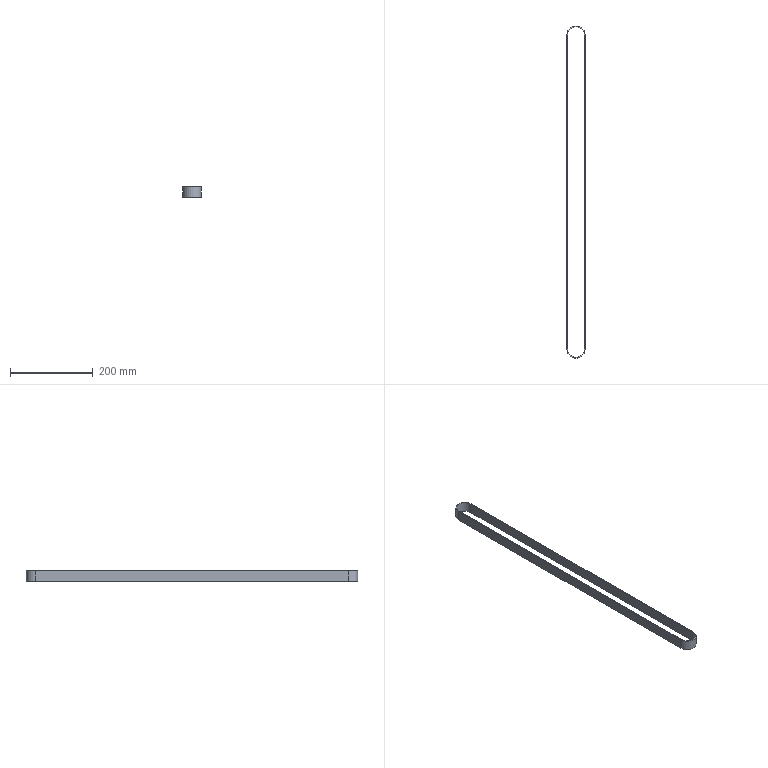Part | SolidWorks | features BaseBody 1 | 1 solid | 10 faces | box 44.42 x 804.42 x 25 mm | volume 82663 mm3 | plane 6 | cylinder 4 | commonest cylinder face diameters 40.42 x2 44.42 x2
STEP:
#1=CARTESIAN_POINT('',(15.21,-745.,-12.5));
#2=VERTEX_POINT('',#1);
#3=CARTESIAN_POINT('',(15.21,15.,-12.5));
#4=VERTEX_POINT('',#3);
#5=CARTESIAN_POINT('',(15.21,15.,-12.5));
#6=DIRECTION('',(0.,1.,0.));
#7=VECTOR('',#6,1000.);
#8=LINE('',#5,#7);
#9=EDGE_CURVE('',#2,#4,#8,.T.);
#10=ORIENTED_EDGE('',*,*,#9,.F.);
#11=CARTESIAN_POINT('',(15.21,-745.,12.5));
#12=VERTEX_POINT('',#11);
#13=CARTESIAN_POINT('',(15.21,-745.,12.5));
#14=DIRECTION('',(0.,0.,-1.));
#15=VECTOR('',#14,1000.);
#16=LINE('',#13,#15);
#17=EDGE_CURVE('',#12,#2,#16,.T.);
#18=ORIENTED_EDGE('',*,*,#17,.F.);
#19=CARTESIAN_POINT('',(15.21,15.,12.5));
#20=VERTEX_POINT('',#19);
#21=CARTESIAN_POINT('',(15.21,15.,12.5));
#22=DIRECTION('',(0.,1.,0.));
#23=VECTOR('',#22,1000.);
#24=LINE('',#21,#23);
#25=EDGE_CURVE('',#12,#20,#24,.T.);
#26=ORIENTED_EDGE('',*,*,#25,.T.);
#27=CARTESIAN_POINT('',(15.21,15.,12.5));
#28=DIRECTION('',(0.,0.,-1.));
#29=VECTOR('',#28,1000.);
#30=LINE('',#27,#29);
#31=EDGE_CURVE('',#20,#4,#30,.T.);
#32=ORIENTED_EDGE('',*,*,#31,.T.);
#33=EDGE_LOOP('',(#10,#18,#26,#32));
#34=FACE_OUTER_BOUND('',#33,.T.);
#35=CARTESIAN_POINT('',(15.21,15.,12.5));
#36=DIRECTION('',(-1.,0.,0.));
#37=DIRECTION('',(0.,0.,1.));
#38=AXIS2_PLACEMENT_3D('',#35,#36,#37);
#39=PLANE('',#38);
#40=ADVANCED_FACE('',(#34),#39,.T.);
#41=CARTESIAN_POINT('',(-25.21,-745.,-12.5));
#42=VERTEX_POINT('',#41);
#43=CARTESIAN_POINT('',(-5.,-745.,-12.5));
#44=DIRECTION('',(0.,0.,1.));
#45=DIRECTION('',(-1.,0.,0.));
#46=AXIS2_PLACEMENT_3D('',#43,#44,#45);
#47=CIRCLE('',#46,20.21);
#48=EDGE_CURVE('',#42,#2,#47,.T.);
#49=ORIENTED_EDGE('',*,*,#48,.F.);
#50=CARTESIAN_POINT('',(-25.21,-745.,12.5));
#51=VERTEX_POINT('',#50);
#52=CARTESIAN_POINT('',(-25.21,-745.,12.5));
#53=DIRECTION('',(0.,0.,-1.));
#54=VECTOR('',#53,1000.);
#55=LINE('',#52,#54);
#56=EDGE_CURVE('',#51,#42,#55,.T.);
#57=ORIENTED_EDGE('',*,*,#56,.F.);
#58=CARTESIAN_POINT('',(-5.,-745.,12.5));
#59=DIRECTION('',(0.,0.,1.));
#60=DIRECTION('',(-1.,0.,0.));
#61=AXIS2_PLACEMENT_3D('',#58,#59,#60);
#62=CIRCLE('',#61,20.21);
#63=EDGE_CURVE('',#51,#12,#62,.T.);
#64=ORIENTED_EDGE('',*,*,#63,.T.);
#65=ORIENTED_EDGE('',*,*,#17,.T.);
#66=EDGE_LOOP('',(#49,#57,#64,#65));
#67=FACE_OUTER_BOUND('',#66,.T.);
#68=CARTESIAN_POINT('',(-5.,-745.,12.5));
#69=DIRECTION('',(0.,0.,-1.));
#70=DIRECTION('',(-1.,0.,0.));
#71=AXIS2_PLACEMENT_3D('',#68,#69,#70);
#72=CYLINDRICAL_SURFACE('',#71,20.21);
#73=ADVANCED_FACE('',(#67),#72,.F.);
#74=CARTESIAN_POINT('',(-25.21,15.,-12.5));
#75=VERTEX_POINT('',#74);
#76=CARTESIAN_POINT('',(-25.21,-745.,-12.5));
#77=DIRECTION('',(0.,-1.,0.));
#78=VECTOR('',#77,1000.);
#79=LINE('',#76,#78);
#80=EDGE_CURVE('',#75,#42,#79,.T.);
#81=ORIENTED_EDGE('',*,*,#80,.F.);
#82=CARTESIAN_POINT('',(-25.21,15.,12.5));
#83=VERTEX_POINT('',#82);
#84=CARTESIAN_POINT('',(-25.21,15.,12.5));
#85=DIRECTION('',(0.,0.,-1.));
#86=VECTOR('',#85,1000.);
#87=LINE('',#84,#86);
#88=EDGE_CURVE('',#83,#75,#87,.T.);
#89=ORIENTED_EDGE('',*,*,#88,.F.);
#90=CARTESIAN_POINT('',(-25.21,-745.,12.5));
#91=DIRECTION('',(0.,-1.,0.));
#92=VECTOR('',#91,1000.);
#93=LINE('',#90,#92);
#94=EDGE_CURVE('',#83,#51,#93,.T.);
#95=ORIENTED_EDGE('',*,*,#94,.T.);
#96=ORIENTED_EDGE('',*,*,#56,.T.);
#97=EDGE_LOOP('',(#81,#89,#95,#96));
#98=FACE_OUTER_BOUND('',#97,.T.);
#99=CARTESIAN_POINT('',(-25.21,-745.,12.5));
#100=DIRECTION('',(1.,0.,0.));
#101=DIRECTION('',(0.,-1.,0.));
#102=AXIS2_PLACEMENT_3D('',#99,#100,#101);
#103=PLANE('',#102);
#104=ADVANCED_FACE('',(#98),#103,.T.);
#105=CARTESIAN_POINT('',(-5.,15.,-12.5));
#106=DIRECTION('',(0.,0.,1.));
#107=DIRECTION('',(-1.,0.,0.));
#108=AXIS2_PLACEMENT_3D('',#105,#106,#107);
#109=CIRCLE('',#108,20.21);
#110=EDGE_CURVE('',#4,#75,#109,.T.);
#111=ORIENTED_EDGE('',*,*,#110,.F.);
#112=ORIENTED_EDGE('',*,*,#31,.F.);
#113=CARTESIAN_POINT('',(-5.,15.,12.5));
#114=DIRECTION('',(0.,0.,1.));
#115=DIRECTION('',(-1.,0.,0.));
#116=AXIS2_PLACEMENT_3D('',#113,#114,#115);
#117=CIRCLE('',#116,20.21);
#118=EDGE_CURVE('',#20,#83,#117,.T.);
#119=ORIENTED_EDGE('',*,*,#118,.T.);
#120=ORIENTED_EDGE('',*,*,#88,.T.);
#121=EDGE_LOOP('',(#111,#112,#119,#120));
#122=FACE_OUTER_BOUND('',#121,.T.);
#123=CARTESIAN_POINT('',(-5.,15.,12.5));
#124=DIRECTION('',(0.,0.,-1.));
#125=DIRECTION('',(-1.,0.,0.));
#126=AXIS2_PLACEMENT_3D('',#123,#124,#125);
#127=CYLINDRICAL_SURFACE('',#126,20.21);
#128=ADVANCED_FACE('',(#122),#127,.F.);
#129=CARTESIAN_POINT('',(17.21,-745.,-12.5));
#130=VERTEX_POINT('',#129);
#131=CARTESIAN_POINT('',(17.21,15.,-12.5));
#132=VERTEX_POINT('',#131);
#133=CARTESIAN_POINT('',(17.21,15.,-12.5));
#134=DIRECTION('',(0.,1.,0.));
#135=VECTOR('',#134,1000.);
#136=LINE('',#133,#135);
#137=EDGE_CURVE('',#130,#132,#136,.T.);
#138=ORIENTED_EDGE('',*,*,#137,.T.);
#139=CARTESIAN_POINT('',(17.21,15.,12.5));
#140=VERTEX_POINT('',#139);
#141=CARTESIAN_POINT('',(17.21,15.,12.5));
#142=DIRECTION('',(0.,0.,-1.));
#143=VECTOR('',#142,1000.);
#144=LINE('',#141,#143);
#145=EDGE_CURVE('',#140,#132,#144,.T.);
#146=ORIENTED_EDGE('',*,*,#145,.F.);
#147=CARTESIAN_POINT('',(17.21,-745.,12.5));
#148=VERTEX_POINT('',#147);
#149=CARTESIAN_POINT('',(17.21,15.,12.5));
#150=DIRECTION('',(0.,1.,0.));
#151=VECTOR('',#150,1000.);
#152=LINE('',#149,#151);
#153=EDGE_CURVE('',#148,#140,#152,.T.);
#154=ORIENTED_EDGE('',*,*,#153,.F.);
#155=CARTESIAN_POINT('',(17.21,-745.,12.5));
#156=DIRECTION('',(0.,0.,-1.));
#157=VECTOR('',#156,1000.);
#158=LINE('',#155,#157);
#159=EDGE_CURVE('',#148,#130,#158,.T.);
#160=ORIENTED_EDGE('',*,*,#159,.T.);
#161=EDGE_LOOP('',(#138,#146,#154,#160));
#162=FACE_OUTER_BOUND('',#161,.T.);
#163=CARTESIAN_POINT('',(17.21,15.,12.5));
#164=DIRECTION('',(-1.,0.,0.));
#165=DIRECTION('',(0.,0.,1.));
#166=AXIS2_PLACEMENT_3D('',#163,#164,#165);
#167=PLANE('',#166);
#168=ADVANCED_FACE('',(#162),#167,.F.);
#169=CARTESIAN_POINT('',(-27.21,-745.,-12.5));
#170=VERTEX_POINT('',#169);
#171=CARTESIAN_POINT('',(-5.,-745.,-12.5));
#172=DIRECTION('',(0.,0.,1.));
#173=DIRECTION('',(-1.,0.,0.));
#174=AXIS2_PLACEMENT_3D('',#171,#172,#173);
#175=CIRCLE('',#174,22.21);
#176=EDGE_CURVE('',#170,#130,#175,.T.);
#177=ORIENTED_EDGE('',*,*,#176,.T.);
#178=ORIENTED_EDGE('',*,*,#159,.F.);
#179=CARTESIAN_POINT('',(-27.21,-745.,12.5));
#180=VERTEX_POINT('',#179);
#181=CARTESIAN_POINT('',(-5.,-745.,12.5));
#182=DIRECTION('',(0.,0.,1.));
#183=DIRECTION('',(-1.,0.,0.));
#184=AXIS2_PLACEMENT_3D('',#181,#182,#183);
#185=CIRCLE('',#184,22.21);
#186=EDGE_CURVE('',#180,#148,#185,.T.);
#187=ORIENTED_EDGE('',*,*,#186,.F.);
#188=CARTESIAN_POINT('',(-27.21,-745.,12.5));
#189=DIRECTION('',(0.,0.,-1.));
#190=VECTOR('',#189,1000.);
#191=LINE('',#188,#190);
#192=EDGE_CURVE('',#180,#170,#191,.T.);
#193=ORIENTED_EDGE('',*,*,#192,.T.);
#194=EDGE_LOOP('',(#177,#178,#187,#193));
#195=FACE_OUTER_BOUND('',#194,.T.);
#196=CARTESIAN_POINT('',(-5.,-745.,12.5));
#197=DIRECTION('',(0.,0.,-1.));
#198=DIRECTION('',(-1.,0.,0.));
#199=AXIS2_PLACEMENT_3D('',#196,#197,#198);
#200=CYLINDRICAL_SURFACE('',#199,22.21);
#201=ADVANCED_FACE('',(#195),#200,.T.);
#202=CARTESIAN_POINT('',(-27.21,15.,-12.5));
#203=VERTEX_POINT('',#202);
#204=CARTESIAN_POINT('',(-27.21,15.,-12.5));
#205=DIRECTION('',(0.,-1.,0.));
#206=VECTOR('',#205,1000.);
#207=LINE('',#204,#206);
#208=EDGE_CURVE('',#203,#170,#207,.T.);
#209=ORIENTED_EDGE('',*,*,#208,.T.);
#210=ORIENTED_EDGE('',*,*,#192,.F.);
#211=CARTESIAN_POINT('',(-27.21,15.,12.5));
#212=VERTEX_POINT('',#211);
#213=CARTESIAN_POINT('',(-27.21,15.,12.5));
#214=DIRECTION('',(0.,-1.,0.));
#215=VECTOR('',#214,1000.);
#216=LINE('',#213,#215);
#217=EDGE_CURVE('',#212,#180,#216,.T.);
#218=ORIENTED_EDGE('',*,*,#217,.F.);
#219=CARTESIAN_POINT('',(-27.21,15.,12.5));
#220=DIRECTION('',(0.,0.,-1.));
#221=VECTOR('',#220,1000.);
#222=LINE('',#219,#221);
#223=EDGE_CURVE('',#212,#203,#222,.T.);
#224=ORIENTED_EDGE('',*,*,#223,.T.);
#225=EDGE_LOOP('',(#209,#210,#218,#224));
#226=FACE_OUTER_BOUND('',#225,.T.);
#227=CARTESIAN_POINT('',(-27.21,15.,12.5));
#228=DIRECTION('',(1.,0.,0.));
#229=DIRECTION('',(0.,-1.,0.));
#230=AXIS2_PLACEMENT_3D('',#227,#228,#229);
#231=PLANE('',#230);
#232=ADVANCED_FACE('',(#226),#231,.F.);
#233=CARTESIAN_POINT('',(-5.,15.,-12.5));
#234=DIRECTION('',(0.,0.,1.));
#235=DIRECTION('',(-1.,0.,0.));
#236=AXIS2_PLACEMENT_3D('',#233,#234,#235);
#237=CIRCLE('',#236,22.21);
#238=EDGE_CURVE('',#132,#203,#237,.T.);
#239=ORIENTED_EDGE('',*,*,#238,.T.);
#240=ORIENTED_EDGE('',*,*,#223,.F.);
#241=CARTESIAN_POINT('',(-5.,15.,12.5));
#242=DIRECTION('',(0.,0.,1.));
#243=DIRECTION('',(-1.,0.,0.));
#244=AXIS2_PLACEMENT_3D('',#241,#242,#243);
#245=CIRCLE('',#244,22.21);
#246=EDGE_CURVE('',#140,#212,#245,.T.);
#247=ORIENTED_EDGE('',*,*,#246,.F.);
#248=ORIENTED_EDGE('',*,*,#145,.T.);
#249=EDGE_LOOP('',(#239,#240,#247,#248));
#250=FACE_OUTER_BOUND('',#249,.T.);
#251=CARTESIAN_POINT('',(-5.,15.,12.5));
#252=DIRECTION('',(0.,0.,-1.));
#253=DIRECTION('',(-1.,0.,0.));
#254=AXIS2_PLACEMENT_3D('',#251,#252,#253);
#255=CYLINDRICAL_SURFACE('',#254,22.21);
#256=ADVANCED_FACE('',(#250),#255,.T.);
#257=ORIENTED_EDGE('',*,*,#9,.T.);
#258=ORIENTED_EDGE('',*,*,#110,.T.);
#259=ORIENTED_EDGE('',*,*,#80,.T.);
#260=ORIENTED_EDGE('',*,*,#48,.T.);
#261=EDGE_LOOP('',(#257,#258,#259,#260));
#262=FACE_BOUND('',#261,.T.);
#263=ORIENTED_EDGE('',*,*,#238,.F.);
#264=ORIENTED_EDGE('',*,*,#137,.F.);
#265=ORIENTED_EDGE('',*,*,#176,.F.);
#266=ORIENTED_EDGE('',*,*,#208,.F.);
#267=EDGE_LOOP('',(#263,#264,#265,#266));
#268=FACE_OUTER_BOUND('',#267,.T.);
#269=CARTESIAN_POINT('',(-5.,15.,-12.5));
#270=DIRECTION('',(0.,0.,-1.));
#271=DIRECTION('',(0.,-1.,0.));
#272=AXIS2_PLACEMENT_3D('',#269,#270,#271);
#273=PLANE('',#272);
#274=ADVANCED_FACE('',(#262,#268),#273,.T.);
#275=ORIENTED_EDGE('',*,*,#118,.F.);
#276=ORIENTED_EDGE('',*,*,#25,.F.);
#277=ORIENTED_EDGE('',*,*,#63,.F.);
#278=ORIENTED_EDGE('',*,*,#94,.F.);
#279=EDGE_LOOP('',(#275,#276,#277,#278));
#280=FACE_BOUND('',#279,.T.);
#281=ORIENTED_EDGE('',*,*,#246,.T.);
#282=ORIENTED_EDGE('',*,*,#217,.T.);
#283=ORIENTED_EDGE('',*,*,#186,.T.);
#284=ORIENTED_EDGE('',*,*,#153,.T.);
#285=EDGE_LOOP('',(#281,#282,#283,#284));
#286=FACE_OUTER_BOUND('',#285,.T.);
#287=CARTESIAN_POINT('',(-5.,15.,12.5));
#288=DIRECTION('',(0.,0.,-1.));
#289=DIRECTION('',(0.,-1.,0.));
#290=AXIS2_PLACEMENT_3D('',#287,#288,#289);
#291=PLANE('',#290);
#292=ADVANCED_FACE('',(#280,#286),#291,.F.);
#293=CLOSED_SHELL('',(#40,#73,#104,#128,#168,#201,#232,#256,#274,#292));
#294=MANIFOLD_SOLID_BREP('',#293);
#295=CARTESIAN_POINT('',(0.,0.,0.));
#296=DIRECTION('',(0.,0.,1.));
#297=DIRECTION('',(1.,0.,0.));
#298=AXIS2_PLACEMENT_3D('',#295,#296,#297);
#299=(LENGTH_UNIT()NAMED_UNIT(*)SI_UNIT(.MILLI.,.METRE.));
#300=UNCERTAINTY_MEASURE_WITH_UNIT(LENGTH_MEASURE(0.00001),#299,'','');
#301=(NAMED_UNIT(*)PLANE_ANGLE_UNIT()SI_UNIT($,.RADIAN.));
#302=(NAMED_UNIT(*)SI_UNIT($,.STERADIAN.)SOLID_ANGLE_UNIT());
#303=(GEOMETRIC_REPRESENTATION_CONTEXT(3)GLOBAL_UNCERTAINTY_ASSIGNED_CONTEXT((#300))GLOBAL_UNIT_ASSIGNED_CONTEXT((#299,#301,#302))REPRESENTATION_CONTEXT('',''));
#304=ADVANCED_BREP_SHAPE_REPRESENTATION('',(#294,#298),#303);